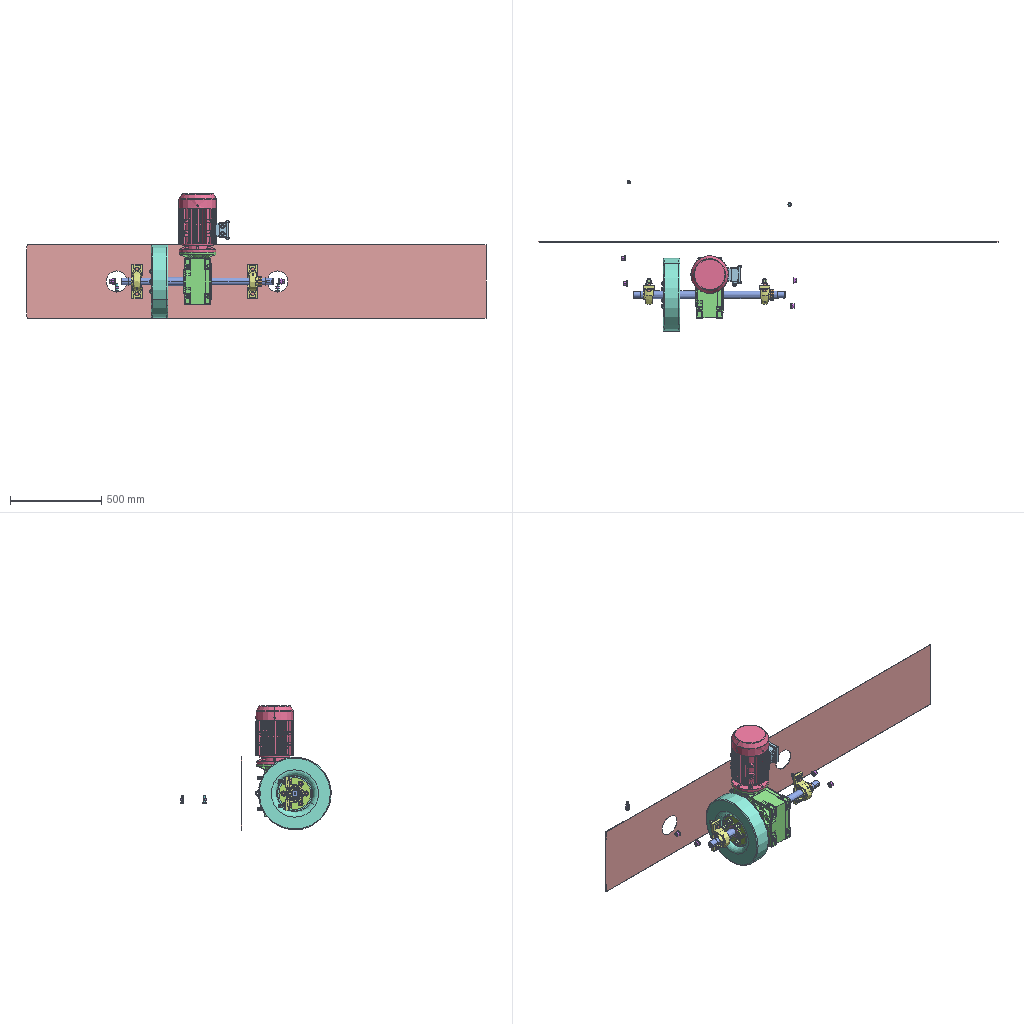Assembly | SolidWorks | 22 different items | 81 placed | box 2516 x 824 x 679 mm
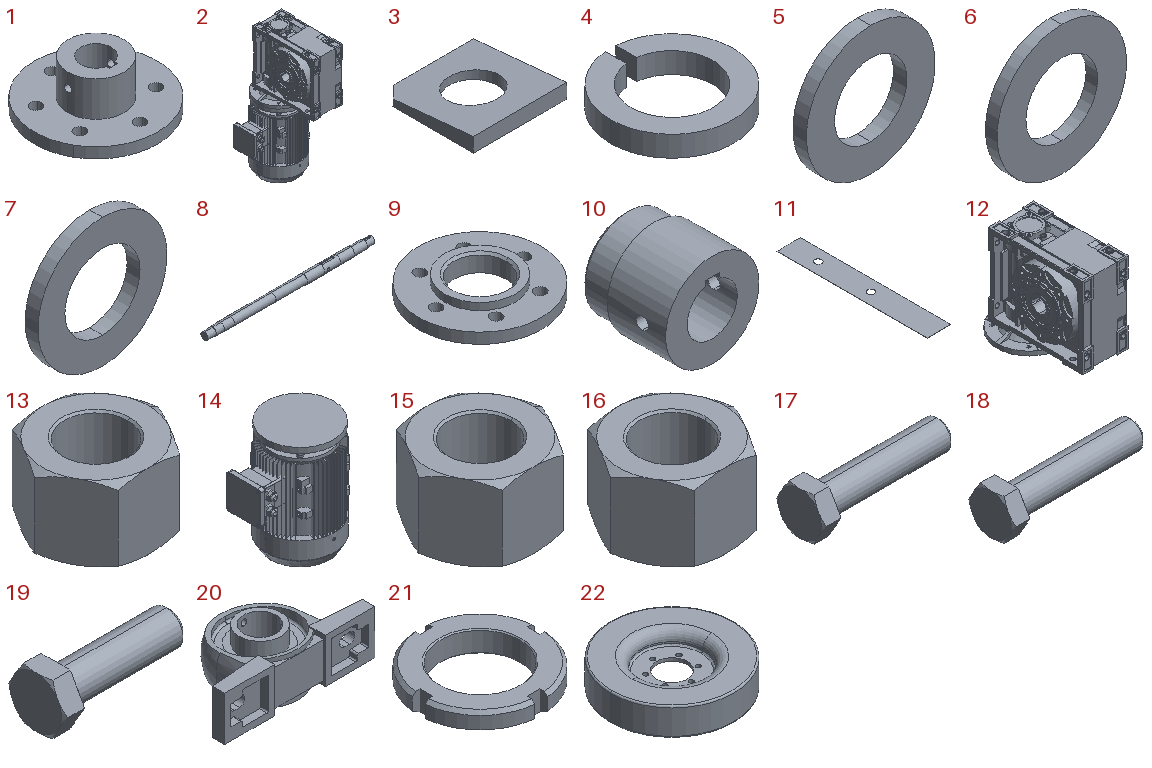Parts list (item | name | quantity | parent item | size | volume | features):
1 | (subassembly) | x1 | - | 175 x 175 x 75 mm | 555297 mm3 | -
2 | (subassembly) | x1 | - | 274.826 x 342.025 x 605.25 mm | 17102127 mm3 | -
3 | - | x4 | - | 35 x 35 x 5.4 mm | 3571 mm3 | features Cut 2, Extrusion 1
4 | - | x4 | - | 21.361 x 21.323 x 3.6 mm | 696.819 mm3 | features Extrusion 1
5 | - | x4 | - | 24 x 2.5 x 24 mm | 773.126 mm3 | features Revolution 1
6 | - | x6 | - | 28 x 2.5 x 28 mm | 1068 mm3 | features Revolution 1
7 | - | x4 | - | 30 x 3 x 30 mm | 1399 mm3 | features Revolution 1
8 | - | x1 | - | 830 x 45 x 45 mm | 1090554 mm3 | features ICE 5, HoleWzd 2, Chamfer 1, MirrorPattern 1, Revolution 1
9 | - | x1 | in 1 | 175 x 175 x 25 mm | 312641 mm3 | features ICE 2, Chamfer 1, Extrusion 1, HoleWzd 1
10 | - | x1 | in 1 | 80 x 75 x 80 mm | 242656 mm3 | features Chamfer 1, HoleWzd 1, ICE 1, Revolution 1
11 | - | x1 | - | 400 x 2517 x 2.5 mm | 2462842 mm3 | features Extrusion 1
12 | - | x1 | in 2 | 200 x 338.5 x 285.25 mm | 8295656 mm3 | features ICE 74, CirPattern 10, Chamfer 9, MirrorPattern 9, Revolution 5, DeleteBody 4, Fillet 3, MirrorSolid 2, Extrusion 1, LPattern 1, PLine 1, Rib 1
13 | - | x16 | - | 22.8 x 19.745 x 13.9 mm | 3143 mm3 | features Cut 2, Chamfer 1, Extrusion 1
14 | - | x1 | in 2 | 274.826 x 207.05 x 320 mm | 8806469 mm3 | features ICE 28, Fillet 9, MirrorPattern 5, CirPattern 4, DeleteBody 4, Chamfer 2, Revolution 2, Extrusion 1, MirrorSolid 1, RevCut 1, SketchPattern 1
15 | - | x10 | - | 19.9 x 17.234 x 12.2 mm | 2145 mm3 | features Cut 2, Chamfer 1, Extrusion 1
16 | - | x4 | - | 26.2 x 22.69 x 15.9 mm | 4666 mm3 | features Cut 2, Chamfer 1, Extrusion 1
17 | - | x10 | - | 68.8 x 24.249 x 21 mm | 12486 mm3 | features RevCut 4, Revolution 2, Chamfer 1, Extrusion 1, LPattern 1
18 | - | x4 | - | 62.5 x 20.785 x 18 mm | 8250 mm3 | features RevCut 4, Revolution 2, Chamfer 1, Extrusion 1, LPattern 1
19 | - | x2 | - | 47.5 x 20.785 x 18 mm | 6554 mm3 | features RevCut 4, Revolution 2, Chamfer 1, Extrusion 1, LPattern 1
20 | - | x2 | - | 186 x 100.8 x 57.7 mm | 292850 mm3 | features Revolution 5, Boss 3, Cut 3, CirPattern 2, RevCut 2, Extrusion 1, RefAxis 1, SweepCut 1
21 | - | x2 | - | 57.689 x 57.689 x 10 mm | 13482 mm3 | features Chamfer 3, CirPattern 1, Cut 1, Extrusion 1
22 | - | x1 | - | 400 x 400 x 90 mm | 8442297 mm3 | features Fillet 1, HoleWzd 1, Revolution 1
Mates (type | each side: item.copy, entity, surface, feature):
In the top assembly
Coincident | 11.1 plane | assembly plane
Coincident | 20.1 face plane Boss-Extrude1 | 20.2 face plane Boss-Extrude1
Concentric | 20.1 face cylinder Boss-Revolve5 | 20.2 face cylinder Boss-Revolve5
Concentric | 8.1 face cylinder Revolve1 | 20.2 face cylinder Boss-Revolve5
Coincident | 8.1 face plane Revolve1 | 20.1 face plane Boss-Revolve5
Coincident | 16.1 face plane Boss-Extrude | 7.1 face plane Boss-Revolve
Parallel | 16.1 face plane Boss-Extrude | assembly plane
Coincident | 16.2 face plane Boss-Extrude | 7.2 face plane Boss-Revolve
Concentric | 16.2 face cylinder Boss-Extrude | 7.2 face cylinder Boss-Revolve
Parallel | 17.1 face plane Boss-Extrude | 13.1 face plane Boss-Extrude
Parallel | 20.2 face plane Boss-Extrude1 | 17.1 face plane Boss-Extrude
Parallel | 17.2 face plane Boss-Extrude | 13.2 face plane Boss-Extrude
Concentric | 17.2 face cylinder Boss-Revolve1 | 4.1 face cylinder Extrude1
Concentric | 17.2 face cylinder Boss-Revolve1 | 13.2 face cylinder Boss-Extrude
Concentric | 17.2 face cylinder Boss-Revolve1 | 3.1 face cylinder Boss-Extrude
Parallel | 3.2 face plane Boss-Extrude | 3.1 face plane Boss-Extrude
Coincident | 3.2 face plane Boss-Extrude | 3.1 face plane Boss-Extrude
Concentric | 8.1 face cylinder Revolve1 | 10.1 face cylinder Revolve1
Coincident | 8.1 face plane Revolve1 | 10.1 face plane Revolve1
Concentric | 8.1 face cylinder Cut-Extrude5 | 10.1 face cylinder M12 Tapped Hole1
Concentric | 16.3 face cylinder Boss-Extrude | 7.3 face cylinder Boss-Revolve
Coincident | 16.3 face plane Boss-Extrude | 7.3 face plane Boss-Revolve
Parallel | 16.2 face plane Boss-Extrude | 16.3 face plane Boss-Extrude
Concentric | 16.4 face cylinder Boss-Extrude | 7.4 face cylinder Boss-Revolve
Coincident | 16.4 face plane Boss-Extrude | 7.4 face plane Boss-Revolve
Concentric | 17.3 face cylinder Boss-Revolve1 | 13.3 face cylinder Boss-Extrude
Concentric | 17.3 face cylinder Boss-Revolve1 | 6.1 face cylinder Boss-Revolve
Parallel | 13.4 face plane Boss-Extrude | 17.4 face plane Boss-Extrude
Concentric | 8.1 face cylinder Revolve1 | 21.1 face cylinder Boss-Extrude
Concentric | 8.1 face cylinder Revolve1 | 21.2 face cylinder Boss-Extrude
Coincident | 21.1 face plane Boss-Extrude | 21.2 face plane Boss-Extrude
Coincident | 20.1 face plane Boss-Revolve5 | 21.1 face plane Boss-Extrude
Parallel | 21.1 face plane CirPattern1 | 21.2 face plane CirPattern1
Parallel | 20.1 face plane Boss-Extrude2 | 21.1 face plane CirPattern1
Parallel | 20.1 face plane Boss-Extrude2 | 13.5 face plane Boss-Extrude
Concentric | 17.3 face cylinder Boss-Revolve1 | 13.6 face cylinder Boss-Extrude
Coincident | 13.3 face plane Boss-Extrude | 13.6 face plane Boss-Extrude | 2 times
Concentric | 19.1 face cylinder Boss-Revolve1 | 15.1 face cylinder Boss-Extrude
Concentric | 19.2 face cylinder Boss-Revolve1 | 15.2 face cylinder Boss-Extrude
Concentric | 8.1 face cylinder Revolve1 | 12.1 face cylinder Boss-Extrude34
Concentric | 18.1 face cylinder Boss-Revolve1 | 15.3 face cylinder Boss-Extrude
Concentric | 18.1 face cylinder Boss-Revolve1 | 15.4 face cylinder Boss-Extrude
Concentric | 18.1 face cylinder Boss-Revolve1 | 5.1 face cylinder Boss-Revolve
Coincident | 15.4 face plane Boss-Extrude | 15.3 face plane Boss-Extrude
Coincident | 5.1 face plane Boss-Revolve | 18.1 face plane Boss-Extrude
Concentric | 12.1 face cylinder Cut-Extrude17 | 18.1 face cylinder Boss-Revolve1
Coincident | 12.1 face plane Cut-Extrude1 | 5.1 face plane Boss-Revolve
Concentric | 8.1 face cylinder Revolve1 | 22.1 face cylinder Revolve1
Concentric | 9.1 face cylinder Ø16.0 (16) Diameter Hole1 | 17.3 face cylinder Boss-Revolve1
Coincident | 9.1 face plane Boss-Extrude2 | 22.1 face plane Revolve1
Coincident | 3.2 face plane Boss-Extrude | 4.2 face plane Extrude1
Coincident | 4.2 face plane Extrude1 | 13.1 face plane Boss-Extrude
Coincident | 20.2 face plane Boss-Extrude2 | 17.1 face plane Boss-Extrude
Coincident | 3.1 face plane Boss-Extrude | 4.1 face plane Extrude1
Coincident | 4.1 face plane Extrude1 | 13.2 face plane Boss-Extrude
Coincident | 20.1 face plane Boss-Extrude2 | 17.2 face plane Boss-Extrude
Coincident | 6.2 face plane Boss-Revolve | 13.4 face plane Boss-Extrude
Coincident | 9.1 face plane Boss-Extrude2 | 6.1 face plane Boss-Revolve
Coincident | 13.3 face plane Boss-Extrude | 6.1 face plane Boss-Revolve
Concentric | 22.1 face cylinder Ø14.5 (14.5) Diameter Hole1 | 17.3 face cylinder Boss-Revolve1
Coincident | 22.1 face plane Revolve1 | 17.4 face plane Boss-Extrude
In subassembly 1
Concentric | 9.2 face cylinder Cut-Extrude1 | 10.2 face cylinder Revolve1
Coincident | 9.2 face plane Boss-Extrude2 | 10.2 face plane Revolve1
Parallel | 10.2 face plane Cut-Extrude1 | 1.1 plane
PlanarAngleDim | 9.2 plane | 1.1 plane
In subassembly 2
Coordinate | 12.2 select_type:25 | 2.1 select_type:11
Coincident | 12.2 face plane Revolve1 | 14.1 face plane Revolve1
Concentric | 12.2 face cylinder Revolve1 | 14.1 face cylinder Revolve1
Coincident | 14.1 plane | 2.1 plane